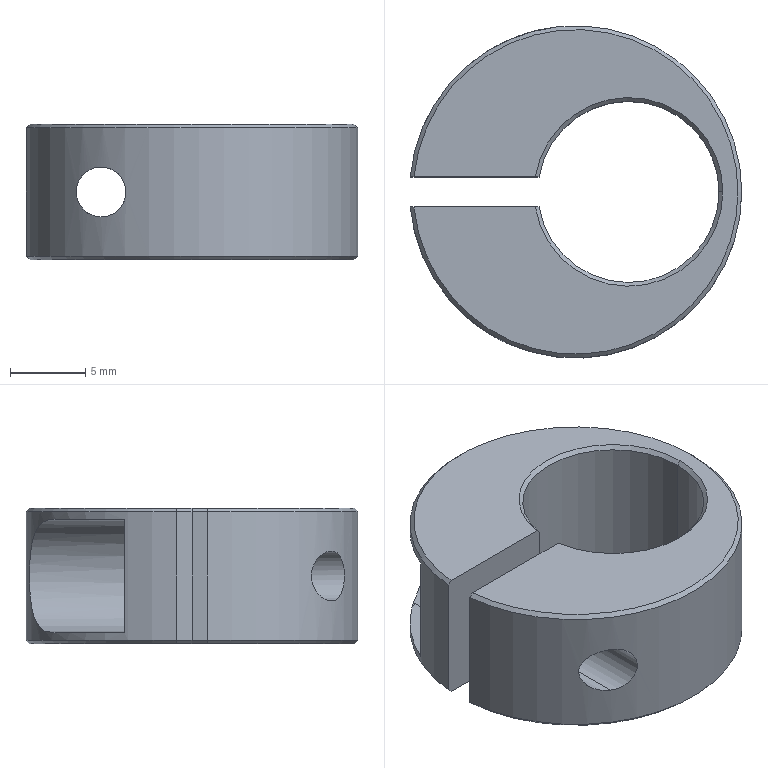Part | NX | features BREP 1 | 1 solid | 25 faces | box 21.954 x 22 x 9 mm | volume 1911 mm3 | cylinder 10 | plane 9 | cone 6 | commonest cylinder face diameters 7.5 x3 3.3 x2 4.5 x2 12 x2 22 x1
STEP:
#1=CARTESIAN_POINT('',(9.5,0.,8.75));
#2=VERTEX_POINT('',#1);
#3=CARTESIAN_POINT('',(9.75,0.,9.));
#4=VERTEX_POINT('',#3);
#5=CARTESIAN_POINT('',(9.5,0.,8.75));
#6=DIRECTION('',(0.7071,0.,0.7071));
#7=VECTOR('',#6,1000.);
#8=LINE('',#5,#7);
#9=EDGE_CURVE('',#2,#4,#8,.T.);
#10=ORIENTED_EDGE('',*,*,#9,.F.);
#11=CARTESIAN_POINT('',(-2.416,-1.,8.75));
#12=VERTEX_POINT('',#11);
#13=CARTESIAN_POINT('',(3.5,0.,8.75));
#14=DIRECTION('',(0.,0.,1.));
#15=DIRECTION('',(1.,0.,0.));
#16=AXIS2_PLACEMENT_3D('',#13,#14,#15);
#17=CIRCLE('',#16,6.);
#18=EDGE_CURVE('',#12,#2,#17,.T.);
#19=ORIENTED_EDGE('',*,*,#18,.F.);
#20=CARTESIAN_POINT('',(-2.669,-1.,9.));
#21=VERTEX_POINT('',#20);
#22=CARTESIAN_POINT('',(-2.669,-1.,9.));
#23=CARTESIAN_POINT('',(-2.585,-1.,8.917));
#24=CARTESIAN_POINT('',(-2.501,-1.,8.833));
#25=CARTESIAN_POINT('',(-2.416,-1.,8.75));
#26=B_SPLINE_CURVE_WITH_KNOTS('',3,(#22,#23,#24,#25),.UNSPECIFIED.,.F.,.F.,(4,4),(0.,0.000356),.UNSPECIFIED.);
#27=EDGE_CURVE('',#21,#12,#26,.T.);
#28=ORIENTED_EDGE('',*,*,#27,.F.);
#29=CARTESIAN_POINT('',(3.5,0.,9.));
#30=DIRECTION('',(0.,0.,-1.));
#31=DIRECTION('',(1.,0.,0.));
#32=AXIS2_PLACEMENT_3D('',#29,#30,#31);
#33=CIRCLE('',#32,6.25);
#34=EDGE_CURVE('',#4,#21,#33,.T.);
#35=ORIENTED_EDGE('',*,*,#34,.F.);
#36=EDGE_LOOP('',(#10,#19,#28,#35));
#37=FACE_BOUND('',#36,.T.);
#38=CARTESIAN_POINT('',(3.5,0.,8.75));
#39=DIRECTION('',(0.,0.,1.));
#40=DIRECTION('',(1.,0.,0.));
#41=AXIS2_PLACEMENT_3D('',#38,#39,#40);
#42=CONICAL_SURFACE('',#41,6.,0.7854);
#43=ADVANCED_FACE('',(#37),#42,.F.);
#44=CARTESIAN_POINT('',(-10.954,-1.,8.75));
#45=VERTEX_POINT('',#44);
#46=CARTESIAN_POINT('',(-10.703,-1.,9.));
#47=VERTEX_POINT('',#46);
#48=CARTESIAN_POINT('',(-10.954,-1.,8.75));
#49=CARTESIAN_POINT('',(-10.871,-1.,8.833));
#50=CARTESIAN_POINT('',(-10.787,-1.,8.917));
#51=CARTESIAN_POINT('',(-10.703,-1.,9.));
#52=B_SPLINE_CURVE_WITH_KNOTS('',3,(#48,#49,#50,#51),.UNSPECIFIED.,.F.,.F.,(4,4),(0.,0.0003543),.UNSPECIFIED.);
#53=EDGE_CURVE('',#45,#47,#52,.T.);
#54=ORIENTED_EDGE('',*,*,#53,.F.);
#55=CARTESIAN_POINT('',(-10.954,1.,8.75));
#56=VERTEX_POINT('',#55);
#57=CARTESIAN_POINT('',(0.,0.,8.75));
#58=DIRECTION('',(0.,0.,-1.));
#59=DIRECTION('',(1.,0.,0.));
#60=AXIS2_PLACEMENT_3D('',#57,#58,#59);
#61=CIRCLE('',#60,11.);
#62=EDGE_CURVE('',#56,#45,#61,.T.);
#63=ORIENTED_EDGE('',*,*,#62,.F.);
#64=CARTESIAN_POINT('',(-10.703,1.,9.));
#65=VERTEX_POINT('',#64);
#66=CARTESIAN_POINT('',(-10.703,1.,9.));
#67=CARTESIAN_POINT('',(-10.787,1.,8.917));
#68=CARTESIAN_POINT('',(-10.871,1.,8.833));
#69=CARTESIAN_POINT('',(-10.954,1.,8.75));
#70=B_SPLINE_CURVE_WITH_KNOTS('',3,(#66,#67,#68,#69),.UNSPECIFIED.,.F.,.F.,(4,4),(0.,0.0003543),.UNSPECIFIED.);
#71=EDGE_CURVE('',#65,#56,#70,.T.);
#72=ORIENTED_EDGE('',*,*,#71,.F.);
#73=CARTESIAN_POINT('',(0.,0.,9.));
#74=DIRECTION('',(0.,0.,1.));
#75=DIRECTION('',(1.,0.,0.));
#76=AXIS2_PLACEMENT_3D('',#73,#74,#75);
#77=CIRCLE('',#76,10.75);
#78=EDGE_CURVE('',#47,#65,#77,.T.);
#79=ORIENTED_EDGE('',*,*,#78,.F.);
#80=EDGE_LOOP('',(#54,#63,#72,#79));
#81=FACE_BOUND('',#80,.T.);
#82=CARTESIAN_POINT('',(0.,0.,9.));
#83=DIRECTION('',(0.,0.,-1.));
#84=DIRECTION('',(-1.,0.,0.));
#85=AXIS2_PLACEMENT_3D('',#82,#83,#84);
#86=CONICAL_SURFACE('',#85,10.75,0.7854);
#87=ADVANCED_FACE('',(#81),#86,.T.);
#88=CARTESIAN_POINT('',(-2.669,1.,0.));
#89=VERTEX_POINT('',#88);
#90=CARTESIAN_POINT('',(-2.416,1.,0.25));
#91=VERTEX_POINT('',#90);
#92=CARTESIAN_POINT('',(-2.669,1.,0.));
#93=CARTESIAN_POINT('',(-2.585,1.,0.08336));
#94=CARTESIAN_POINT('',(-2.501,1.,0.1667));
#95=CARTESIAN_POINT('',(-2.416,1.,0.25));
#96=B_SPLINE_CURVE_WITH_KNOTS('',3,(#92,#93,#94,#95),.UNSPECIFIED.,.F.,.F.,(4,4),(0.,0.000356),.UNSPECIFIED.);
#97=EDGE_CURVE('',#89,#91,#96,.T.);
#98=ORIENTED_EDGE('',*,*,#97,.F.);
#99=CARTESIAN_POINT('',(-2.669,-1.,0.));
#100=VERTEX_POINT('',#99);
#101=CARTESIAN_POINT('',(3.5,0.,0.));
#102=DIRECTION('',(0.,0.,1.));
#103=DIRECTION('',(1.,0.,0.));
#104=AXIS2_PLACEMENT_3D('',#101,#102,#103);
#105=CIRCLE('',#104,6.25);
#106=EDGE_CURVE('',#100,#89,#105,.T.);
#107=ORIENTED_EDGE('',*,*,#106,.F.);
#108=CARTESIAN_POINT('',(-2.416,-1.,0.25));
#109=VERTEX_POINT('',#108);
#110=CARTESIAN_POINT('',(-2.416,-1.,0.25));
#111=CARTESIAN_POINT('',(-2.501,-1.,0.1667));
#112=CARTESIAN_POINT('',(-2.585,-1.,0.08336));
#113=CARTESIAN_POINT('',(-2.669,-1.,0.));
#114=B_SPLINE_CURVE_WITH_KNOTS('',3,(#110,#111,#112,#113),.UNSPECIFIED.,.F.,.F.,(4,4),(0.,0.000356),.UNSPECIFIED.);
#115=EDGE_CURVE('',#109,#100,#114,.T.);
#116=ORIENTED_EDGE('',*,*,#115,.F.);
#117=CARTESIAN_POINT('',(9.5,0.,0.25));
#118=VERTEX_POINT('',#117);
#119=CARTESIAN_POINT('',(3.5,0.,0.25));
#120=DIRECTION('',(0.,0.,-1.));
#121=DIRECTION('',(1.,0.,0.));
#122=AXIS2_PLACEMENT_3D('',#119,#120,#121);
#123=CIRCLE('',#122,6.);
#124=EDGE_CURVE('',#118,#109,#123,.T.);
#125=ORIENTED_EDGE('',*,*,#124,.F.);
#126=CARTESIAN_POINT('',(3.5,0.,0.25));
#127=DIRECTION('',(0.,0.,-1.));
#128=DIRECTION('',(1.,0.,0.));
#129=AXIS2_PLACEMENT_3D('',#126,#127,#128);
#130=CIRCLE('',#129,6.);
#131=EDGE_CURVE('',#91,#118,#130,.T.);
#132=ORIENTED_EDGE('',*,*,#131,.F.);
#133=EDGE_LOOP('',(#98,#107,#116,#125,#132));
#134=FACE_BOUND('',#133,.T.);
#135=CARTESIAN_POINT('',(3.5,0.,0.25));
#136=DIRECTION('',(0.,0.,-1.));
#137=DIRECTION('',(-1.,0.,0.));
#138=AXIS2_PLACEMENT_3D('',#135,#136,#137);
#139=CONICAL_SURFACE('',#138,6.,0.7854);
#140=ADVANCED_FACE('',(#134),#139,.F.);
#141=CARTESIAN_POINT('',(10.75,0.,0.));
#142=VERTEX_POINT('',#141);
#143=CARTESIAN_POINT('',(11.,0.,0.25));
#144=VERTEX_POINT('',#143);
#145=CARTESIAN_POINT('',(11.,0.,0.25));
#146=DIRECTION('',(0.7071,0.,0.7071));
#147=VECTOR('',#146,1000.);
#148=LINE('',#145,#147);
#149=EDGE_CURVE('',#142,#144,#148,.T.);
#150=ORIENTED_EDGE('',*,*,#149,.F.);
#151=CARTESIAN_POINT('',(-10.703,1.,0.));
#152=VERTEX_POINT('',#151);
#153=CARTESIAN_POINT('',(0.,0.,0.));
#154=DIRECTION('',(0.,0.,-1.));
#155=DIRECTION('',(1.,0.,0.));
#156=AXIS2_PLACEMENT_3D('',#153,#154,#155);
#157=CIRCLE('',#156,10.75);
#158=EDGE_CURVE('',#152,#142,#157,.T.);
#159=ORIENTED_EDGE('',*,*,#158,.F.);
#160=CARTESIAN_POINT('',(-10.954,1.,0.25));
#161=VERTEX_POINT('',#160);
#162=CARTESIAN_POINT('',(-10.954,1.,0.25));
#163=CARTESIAN_POINT('',(-10.871,1.,0.1667));
#164=CARTESIAN_POINT('',(-10.787,1.,0.08333));
#165=CARTESIAN_POINT('',(-10.703,1.,0.));
#166=B_SPLINE_CURVE_WITH_KNOTS('',3,(#162,#163,#164,#165),.UNSPECIFIED.,.F.,.F.,(4,4),(0.,0.0003543),.UNSPECIFIED.);
#167=EDGE_CURVE('',#161,#152,#166,.T.);
#168=ORIENTED_EDGE('',*,*,#167,.F.);
#169=CARTESIAN_POINT('',(0.,0.,0.25));
#170=DIRECTION('',(0.,0.,1.));
#171=DIRECTION('',(1.,0.,0.));
#172=AXIS2_PLACEMENT_3D('',#169,#170,#171);
#173=CIRCLE('',#172,11.);
#174=EDGE_CURVE('',#144,#161,#173,.T.);
#175=ORIENTED_EDGE('',*,*,#174,.F.);
#176=EDGE_LOOP('',(#150,#159,#168,#175));
#177=FACE_BOUND('',#176,.T.);
#178=CARTESIAN_POINT('',(0.,0.,0.25));
#179=DIRECTION('',(0.,0.,1.));
#180=DIRECTION('',(1.,0.,0.));
#181=AXIS2_PLACEMENT_3D('',#178,#179,#180);
#182=CONICAL_SURFACE('',#181,11.,0.7854);
#183=ADVANCED_FACE('',(#177),#182,.T.);
#184=CARTESIAN_POINT('',(-6.,-1.,2.85));
#185=VERTEX_POINT('',#184);
#186=CARTESIAN_POINT('',(-6.,-9.22,2.85));
#187=VERTEX_POINT('',#186);
#188=CARTESIAN_POINT('',(-6.,-1.,2.85));
#189=DIRECTION('',(0.,1.,0.));
#190=VECTOR('',#189,1000.);
#191=LINE('',#188,#190);
#192=EDGE_CURVE('',#185,#187,#191,.F.);
#193=ORIENTED_EDGE('',*,*,#192,.T.);
#194=CARTESIAN_POINT('',(-6.,-9.22,6.15));
#195=VERTEX_POINT('',#194);
#196=CARTESIAN_POINT('',(-6.,-9.22,2.85));
#197=CARTESIAN_POINT('',(-5.573,-9.497,2.85));
#198=CARTESIAN_POINT('',(-4.796,-9.917,3.131));
#199=CARTESIAN_POINT('',(-4.125,-10.197,4.506));
#200=CARTESIAN_POINT('',(-4.804,-9.914,5.873));
#201=CARTESIAN_POINT('',(-5.574,-9.496,6.15));
#202=CARTESIAN_POINT('',(-6.,-9.22,6.15));
#203=B_SPLINE_CURVE_WITH_KNOTS('',3,(#196,#197,#198,#199,#200,#201,#202),.UNSPECIFIED.,.F.,.F.,(4,1,1,1,4),(0.,0.25,0.5,0.75,1.),.UNSPECIFIED.);
#204=EDGE_CURVE('',#195,#187,#203,.F.);
#205=ORIENTED_EDGE('',*,*,#204,.F.);
#206=CARTESIAN_POINT('',(-6.,-1.,6.15));
#207=VERTEX_POINT('',#206);
#208=CARTESIAN_POINT('',(-6.,-1.,6.15));
#209=DIRECTION('',(0.,1.,0.));
#210=VECTOR('',#209,1000.);
#211=LINE('',#208,#210);
#212=EDGE_CURVE('',#207,#195,#211,.F.);
#213=ORIENTED_EDGE('',*,*,#212,.F.);
#214=CARTESIAN_POINT('',(-6.,-1.,4.5));
#215=DIRECTION('',(0.,1.,0.));
#216=DIRECTION('',(0.,0.,1.));
#217=AXIS2_PLACEMENT_3D('',#214,#215,#216);
#218=CIRCLE('',#217,1.65);
#219=EDGE_CURVE('',#207,#185,#218,.T.);
#220=ORIENTED_EDGE('',*,*,#219,.T.);
#221=EDGE_LOOP('',(#193,#205,#213,#220));
#222=FACE_BOUND('',#221,.T.);
#223=CARTESIAN_POINT('',(-6.,-1.,4.5));
#224=DIRECTION('',(0.,1.,0.));
#225=DIRECTION('',(0.,0.,1.));
#226=AXIS2_PLACEMENT_3D('',#223,#224,#225);
#227=CYLINDRICAL_SURFACE('',#226,1.65);
#228=ADVANCED_FACE('',(#222),#227,.F.);
#229=CARTESIAN_POINT('',(-6.325,9.,8.25));
#230=VERTEX_POINT('',#229);
#231=CARTESIAN_POINT('',(-6.325,9.,8.236));
#232=VERTEX_POINT('',#231);
#233=CARTESIAN_POINT('',(-6.325,9.,9.));
#234=DIRECTION('',(0.,0.,-1.));
#235=VECTOR('',#234,1000.);
#236=LINE('',#233,#235);
#237=EDGE_CURVE('',#230,#232,#236,.T.);
#238=ORIENTED_EDGE('',*,*,#237,.T.);
#239=CARTESIAN_POINT('',(-6.,9.,8.25));
#240=VERTEX_POINT('',#239);
#241=CARTESIAN_POINT('',(-6.,9.,4.5));
#242=DIRECTION('',(0.,1.,0.));
#243=DIRECTION('',(0.,0.,-1.));
#244=AXIS2_PLACEMENT_3D('',#241,#242,#243);
#245=CIRCLE('',#244,3.75);
#246=EDGE_CURVE('',#232,#240,#245,.T.);
#247=ORIENTED_EDGE('',*,*,#246,.T.);
#248=CARTESIAN_POINT('',(-6.,9.,8.25));
#249=DIRECTION('',(1.,0.,0.));
#250=VECTOR('',#249,1000.);
#251=LINE('',#248,#250);
#252=EDGE_CURVE('',#230,#240,#251,.T.);
#253=ORIENTED_EDGE('',*,*,#252,.F.);
#254=EDGE_LOOP('',(#238,#247,#253));
#255=FACE_BOUND('',#254,.T.);
#256=CARTESIAN_POINT('',(0.,9.,0.));
#257=DIRECTION('',(0.,-1.,0.));
#258=DIRECTION('',(0.,0.,-1.));
#259=AXIS2_PLACEMENT_3D('',#256,#257,#258);
#260=PLANE('',#259);
#261=ADVANCED_FACE('',(#255),#260,.T.);
#262=CARTESIAN_POINT('',(-6.325,9.,0.7641));
#263=VERTEX_POINT('',#262);
#264=CARTESIAN_POINT('',(-6.325,9.,0.75));
#265=VERTEX_POINT('',#264);
#266=CARTESIAN_POINT('',(-6.325,9.,9.));
#267=DIRECTION('',(0.,0.,-1.));
#268=VECTOR('',#267,1000.);
#269=LINE('',#266,#268);
#270=EDGE_CURVE('',#263,#265,#269,.T.);
#271=ORIENTED_EDGE('',*,*,#270,.T.);
#272=CARTESIAN_POINT('',(-6.,9.,0.75));
#273=VERTEX_POINT('',#272);
#274=CARTESIAN_POINT('',(-6.,9.,0.75));
#275=DIRECTION('',(-1.,0.,0.));
#276=VECTOR('',#275,1000.);
#277=LINE('',#274,#276);
#278=EDGE_CURVE('',#273,#265,#277,.T.);
#279=ORIENTED_EDGE('',*,*,#278,.F.);
#280=CARTESIAN_POINT('',(-6.,9.,4.5));
#281=DIRECTION('',(0.,1.,0.));
#282=DIRECTION('',(0.,0.,-1.));
#283=AXIS2_PLACEMENT_3D('',#280,#281,#282);
#284=CIRCLE('',#283,3.75);
#285=EDGE_CURVE('',#273,#263,#284,.T.);
#286=ORIENTED_EDGE('',*,*,#285,.T.);
#287=EDGE_LOOP('',(#271,#279,#286));
#288=FACE_BOUND('',#287,.T.);
#289=CARTESIAN_POINT('',(0.,9.,0.));
#290=DIRECTION('',(0.,-1.,0.));
#291=DIRECTION('',(0.,0.,-1.));
#292=AXIS2_PLACEMENT_3D('',#289,#290,#291);
#293=PLANE('',#292);
#294=ADVANCED_FACE('',(#288),#293,.T.);
#295=CARTESIAN_POINT('',(-10.037,4.5,0.75));
#296=VERTEX_POINT('',#295);
#297=CARTESIAN_POINT('',(0.,0.,0.75));
#298=DIRECTION('',(0.,0.,1.));
#299=DIRECTION('',(1.,0.,0.));
#300=AXIS2_PLACEMENT_3D('',#297,#298,#299);
#301=CIRCLE('',#300,11.);
#302=EDGE_CURVE('',#265,#296,#301,.T.);
#303=ORIENTED_EDGE('',*,*,#302,.T.);
#304=CARTESIAN_POINT('',(-6.,4.5,0.75));
#305=VERTEX_POINT('',#304);
#306=CARTESIAN_POINT('',(-6.,4.5,0.75));
#307=DIRECTION('',(-1.,0.,0.));
#308=VECTOR('',#307,1000.);
#309=LINE('',#306,#308);
#310=EDGE_CURVE('',#305,#296,#309,.T.);
#311=ORIENTED_EDGE('',*,*,#310,.F.);
#312=CARTESIAN_POINT('',(-6.,9.,0.75));
#313=DIRECTION('',(0.,-1.,0.));
#314=VECTOR('',#313,1000.);
#315=LINE('',#312,#314);
#316=EDGE_CURVE('',#273,#305,#315,.T.);
#317=ORIENTED_EDGE('',*,*,#316,.F.);
#318=ORIENTED_EDGE('',*,*,#278,.T.);
#319=EDGE_LOOP('',(#303,#311,#317,#318));
#320=FACE_BOUND('',#319,.T.);
#321=CARTESIAN_POINT('',(-6.,9.,0.75));
#322=DIRECTION('',(0.,0.,1.));
#323=DIRECTION('',(1.,0.,0.));
#324=AXIS2_PLACEMENT_3D('',#321,#322,#323);
#325=PLANE('',#324);
#326=ADVANCED_FACE('',(#320),#325,.T.);
#327=CARTESIAN_POINT('',(-10.037,4.5,8.25));
#328=VERTEX_POINT('',#327);
#329=CARTESIAN_POINT('',(0.,0.,8.25));
#330=DIRECTION('',(0.,0.,-1.));
#331=DIRECTION('',(-1.,0.,0.));
#332=AXIS2_PLACEMENT_3D('',#329,#330,#331);
#333=CIRCLE('',#332,11.);
#334=EDGE_CURVE('',#328,#230,#333,.T.);
#335=ORIENTED_EDGE('',*,*,#334,.T.);
#336=ORIENTED_EDGE('',*,*,#252,.T.);
#337=CARTESIAN_POINT('',(-6.,4.5,8.25));
#338=VERTEX_POINT('',#337);
#339=CARTESIAN_POINT('',(-6.,9.,8.25));
#340=DIRECTION('',(0.,-1.,0.));
#341=VECTOR('',#340,1000.);
#342=LINE('',#339,#341);
#343=EDGE_CURVE('',#240,#338,#342,.T.);
#344=ORIENTED_EDGE('',*,*,#343,.T.);
#345=CARTESIAN_POINT('',(-6.,4.5,8.25));
#346=DIRECTION('',(1.,0.,0.));
#347=VECTOR('',#346,1000.);
#348=LINE('',#345,#347);
#349=EDGE_CURVE('',#328,#338,#348,.T.);
#350=ORIENTED_EDGE('',*,*,#349,.F.);
#351=EDGE_LOOP('',(#335,#336,#344,#350));
#352=FACE_BOUND('',#351,.T.);
#353=CARTESIAN_POINT('',(-6.,9.,8.25));
#354=DIRECTION('',(0.,0.,-1.));
#355=DIRECTION('',(-1.,0.,0.));
#356=AXIS2_PLACEMENT_3D('',#353,#354,#355);
#357=PLANE('',#356);
#358=ADVANCED_FACE('',(#352),#357,.T.);
#359=ORIENTED_EDGE('',*,*,#349,.T.);
#360=CARTESIAN_POINT('',(-6.,4.5,4.5));
#361=DIRECTION('',(0.,-1.,0.));
#362=DIRECTION('',(0.,0.,-1.));
#363=AXIS2_PLACEMENT_3D('',#360,#361,#362);
#364=CIRCLE('',#363,3.75);
#365=EDGE_CURVE('',#305,#338,#364,.T.);
#366=ORIENTED_EDGE('',*,*,#365,.F.);
#367=ORIENTED_EDGE('',*,*,#310,.T.);
#368=CARTESIAN_POINT('',(-10.037,4.5,9.));
#369=DIRECTION('',(0.,0.,-1.));
#370=VECTOR('',#369,1000.);
#371=LINE('',#368,#370);
#372=EDGE_CURVE('',#328,#296,#371,.T.);
#373=ORIENTED_EDGE('',*,*,#372,.F.);
#374=EDGE_LOOP('',(#359,#366,#367,#373));
#375=FACE_BOUND('',#374,.T.);
#376=CARTESIAN_POINT('',(-6.,4.5,2.25));
#377=VERTEX_POINT('',#376);
#378=CARTESIAN_POINT('',(-6.,4.5,6.75));
#379=VERTEX_POINT('',#378);
#380=CARTESIAN_POINT('',(-6.,4.5,4.5));
#381=DIRECTION('',(0.,1.,0.));
#382=DIRECTION('',(0.,0.,-1.));
#383=AXIS2_PLACEMENT_3D('',#380,#381,#382);
#384=CIRCLE('',#383,2.25);
#385=EDGE_CURVE('',#377,#379,#384,.T.);
#386=ORIENTED_EDGE('',*,*,#385,.F.);
#387=CARTESIAN_POINT('',(-6.,4.5,4.5));
#388=DIRECTION('',(0.,1.,0.));
#389=DIRECTION('',(0.,0.,-1.));
#390=AXIS2_PLACEMENT_3D('',#387,#388,#389);
#391=CIRCLE('',#390,2.25);
#392=EDGE_CURVE('',#379,#377,#391,.T.);
#393=ORIENTED_EDGE('',*,*,#392,.F.);
#394=EDGE_LOOP('',(#386,#393));
#395=FACE_BOUND('',#394,.T.);
#396=CARTESIAN_POINT('',(-6.,4.5,4.5));
#397=DIRECTION('',(0.,-1.,0.));
#398=DIRECTION('',(0.,0.,-1.));
#399=AXIS2_PLACEMENT_3D('',#396,#397,#398);
#400=PLANE('',#399);
#401=ADVANCED_FACE('',(#375,#395),#400,.F.);
#402=CARTESIAN_POINT('',(-6.,1.,6.75));
#403=VERTEX_POINT('',#402);
#404=CARTESIAN_POINT('',(-6.,4.5,6.75));
#405=DIRECTION('',(0.,-1.,0.));
#406=VECTOR('',#405,1000.);
#407=LINE('',#404,#406);
#408=EDGE_CURVE('',#379,#403,#407,.T.);
#409=ORIENTED_EDGE('',*,*,#408,.F.);
#410=ORIENTED_EDGE('',*,*,#392,.T.);
#411=CARTESIAN_POINT('',(-6.,1.,2.25));
#412=VERTEX_POINT('',#411);
#413=CARTESIAN_POINT('',(-6.,4.5,2.25));
#414=DIRECTION('',(0.,-1.,0.));
#415=VECTOR('',#414,1000.);
#416=LINE('',#413,#415);
#417=EDGE_CURVE('',#377,#412,#416,.T.);
#418=ORIENTED_EDGE('',*,*,#417,.T.);
#419=CARTESIAN_POINT('',(-6.,1.,4.5));
#420=DIRECTION('',(0.,-1.,0.));
#421=DIRECTION('',(0.,0.,-1.));
#422=AXIS2_PLACEMENT_3D('',#419,#420,#421);
#423=CIRCLE('',#422,2.25);
#424=EDGE_CURVE('',#412,#403,#423,.T.);
#425=ORIENTED_EDGE('',*,*,#424,.T.);
#426=EDGE_LOOP('',(#409,#410,#418,#425));
#427=FACE_BOUND('',#426,.T.);
#428=CARTESIAN_POINT('',(-6.,4.5,4.5));
#429=DIRECTION('',(0.,-1.,0.));
#430=DIRECTION('',(0.,0.,-1.));
#431=AXIS2_PLACEMENT_3D('',#428,#429,#430);
#432=CYLINDRICAL_SURFACE('',#431,2.25);
#433=ADVANCED_FACE('',(#427),#432,.F.);
#434=CARTESIAN_POINT('',(-10.703,-1.,0.));
#435=VERTEX_POINT('',#434);
#436=CARTESIAN_POINT('',(-19.584,-1.,0.));
#437=DIRECTION('',(-1.,0.,0.));
#438=VECTOR('',#437,1000.);
#439=LINE('',#436,#438);
#440=EDGE_CURVE('',#100,#435,#439,.T.);
#441=ORIENTED_EDGE('',*,*,#440,.T.);
#442=CARTESIAN_POINT('',(-10.954,-1.,0.25));
#443=VERTEX_POINT('',#442);
#444=CARTESIAN_POINT('',(-10.703,-1.,0.));
#445=CARTESIAN_POINT('',(-10.787,-1.,0.08333));
#446=CARTESIAN_POINT('',(-10.871,-1.,0.1667));
#447=CARTESIAN_POINT('',(-10.954,-1.,0.25));
#448=B_SPLINE_CURVE_WITH_KNOTS('',3,(#444,#445,#446,#447),.UNSPECIFIED.,.F.,.F.,(4,4),(0.,0.0003543),.UNSPECIFIED.);
#449=EDGE_CURVE('',#435,#443,#448,.T.);
#450=ORIENTED_EDGE('',*,*,#449,.T.);
#451=CARTESIAN_POINT('',(-10.954,-1.,9.));
#452=DIRECTION('',(0.,0.,1.));
#453=VECTOR('',#452,1000.);
#454=LINE('',#451,#453);
#455=EDGE_CURVE('',#443,#45,#454,.T.);
#456=ORIENTED_EDGE('',*,*,#455,.T.);
#457=ORIENTED_EDGE('',*,*,#53,.T.);
#458=CARTESIAN_POINT('',(-19.584,-1.,9.));
#459=DIRECTION('',(1.,0.,0.));
#460=VECTOR('',#459,1000.);
#461=LINE('',#458,#460);
#462=EDGE_CURVE('',#47,#21,#461,.T.);
#463=ORIENTED_EDGE('',*,*,#462,.T.);
#464=ORIENTED_EDGE('',*,*,#27,.T.);
#465=CARTESIAN_POINT('',(-2.416,-1.,-0.001));
#466=DIRECTION('',(0.,0.,-1.));
#467=VECTOR('',#466,1000.);
#468=LINE('',#465,#467);
#469=EDGE_CURVE('',#12,#109,#468,.T.);
#470=ORIENTED_EDGE('',*,*,#469,.T.);
#471=ORIENTED_EDGE('',*,*,#115,.T.);
#472=EDGE_LOOP('',(#441,#450,#456,#457,#463,#464,#470,#471));
#473=FACE_BOUND('',#472,.T.);
#474=ORIENTED_EDGE('',*,*,#219,.F.);
#475=CARTESIAN_POINT('',(-6.,-1.,4.5));
#476=DIRECTION('',(0.,1.,0.));
#477=DIRECTION('',(0.,0.,1.));
#478=AXIS2_PLACEMENT_3D('',#475,#476,#477);
#479=CIRCLE('',#478,1.65);
#480=EDGE_CURVE('',#185,#207,#479,.T.);
#481=ORIENTED_EDGE('',*,*,#480,.F.);
#482=EDGE_LOOP('',(#474,#481));
#483=FACE_BOUND('',#482,.T.);
#484=CARTESIAN_POINT('',(-19.584,-1.,-0.001));
#485=DIRECTION('',(0.,-1.,0.));
#486=DIRECTION('',(0.,0.,-1.));
#487=AXIS2_PLACEMENT_3D('',#484,#485,#486);
#488=PLANE('',#487);
#489=ADVANCED_FACE('',(#473,#483),#488,.F.);
#490=CARTESIAN_POINT('',(-10.954,1.,9.));
#491=DIRECTION('',(0.,0.,-1.));
#492=VECTOR('',#491,1000.);
#493=LINE('',#490,#492);
#494=EDGE_CURVE('',#56,#161,#493,.T.);
#495=ORIENTED_EDGE('',*,*,#494,.T.);
#496=ORIENTED_EDGE('',*,*,#167,.T.);
#497=CARTESIAN_POINT('',(-19.584,1.,0.));
#498=DIRECTION('',(1.,0.,0.));
#499=VECTOR('',#498,1000.);
#500=LINE('',#497,#499);
#501=EDGE_CURVE('',#152,#89,#500,.T.);
#502=ORIENTED_EDGE('',*,*,#501,.T.);
#503=ORIENTED_EDGE('',*,*,#97,.T.);
#504=CARTESIAN_POINT('',(-2.416,1.,8.75));
#505=VERTEX_POINT('',#504);
#506=CARTESIAN_POINT('',(-2.416,1.,-0.001));
#507=DIRECTION('',(0.,0.,1.));
#508=VECTOR('',#507,1000.);
#509=LINE('',#506,#508);
#510=EDGE_CURVE('',#91,#505,#509,.T.);
#511=ORIENTED_EDGE('',*,*,#510,.T.);
#512=CARTESIAN_POINT('',(-2.669,1.,9.));
#513=VERTEX_POINT('',#512);
#514=CARTESIAN_POINT('',(-2.416,1.,8.75));
#515=CARTESIAN_POINT('',(-2.501,1.,8.833));
#516=CARTESIAN_POINT('',(-2.585,1.,8.917));
#517=CARTESIAN_POINT('',(-2.669,1.,9.));
#518=B_SPLINE_CURVE_WITH_KNOTS('',3,(#514,#515,#516,#517),.UNSPECIFIED.,.F.,.F.,(4,4),(0.,0.000356),.UNSPECIFIED.);
#519=EDGE_CURVE('',#505,#513,#518,.T.);
#520=ORIENTED_EDGE('',*,*,#519,.T.);
#521=CARTESIAN_POINT('',(-19.584,1.,9.));
#522=DIRECTION('',(-1.,0.,0.));
#523=VECTOR('',#522,1000.);
#524=LINE('',#521,#523);
#525=EDGE_CURVE('',#513,#65,#524,.T.);
#526=ORIENTED_EDGE('',*,*,#525,.T.);
#527=ORIENTED_EDGE('',*,*,#71,.T.);
#528=EDGE_LOOP('',(#495,#496,#502,#503,#511,#520,#526,#527));
#529=FACE_BOUND('',#528,.T.);
#530=ORIENTED_EDGE('',*,*,#424,.F.);
#531=CARTESIAN_POINT('',(-6.,1.,4.5));
#532=DIRECTION('',(0.,-1.,0.));
#533=DIRECTION('',(0.,0.,-1.));
#534=AXIS2_PLACEMENT_3D('',#531,#532,#533);
#535=CIRCLE('',#534,2.25);
#536=EDGE_CURVE('',#403,#412,#535,.T.);
#537=ORIENTED_EDGE('',*,*,#536,.F.);
#538=EDGE_LOOP('',(#530,#537));
#539=FACE_BOUND('',#538,.T.);
#540=CARTESIAN_POINT('',(-19.584,1.,-0.001));
#541=DIRECTION('',(0.,1.,0.));
#542=DIRECTION('',(0.,0.,1.));
#543=AXIS2_PLACEMENT_3D('',#540,#541,#542);
#544=PLANE('',#543);
#545=ADVANCED_FACE('',(#529,#539),#544,.F.);
#546=CARTESIAN_POINT('',(9.5,0.,-0.001));
#547=DIRECTION('',(0.,0.,1.));
#548=VECTOR('',#547,1000.);
#549=LINE('',#546,#548);
#550=EDGE_CURVE('',#118,#2,#549,.T.);
#551=ORIENTED_EDGE('',*,*,#550,.F.);
#552=ORIENTED_EDGE('',*,*,#124,.T.);
#553=ORIENTED_EDGE('',*,*,#469,.F.);
#554=ORIENTED_EDGE('',*,*,#18,.T.);
#555=EDGE_LOOP('',(#551,#552,#553,#554));
#556=FACE_BOUND('',#555,.T.);
#557=CARTESIAN_POINT('',(3.5,0.,-0.001));
#558=DIRECTION('',(0.,0.,1.));
#559=DIRECTION('',(1.,0.,0.));
#560=AXIS2_PLACEMENT_3D('',#557,#558,#559);
#561=CYLINDRICAL_SURFACE('',#560,6.);
#562=ADVANCED_FACE('',(#556),#561,.F.);
#563=ORIENTED_EDGE('',*,*,#501,.F.);
#564=ORIENTED_EDGE('',*,*,#158,.T.);
#565=CARTESIAN_POINT('',(0.,0.,0.));
#566=DIRECTION('',(0.,0.,-1.));
#567=DIRECTION('',(1.,0.,0.));
#568=AXIS2_PLACEMENT_3D('',#565,#566,#567);
#569=CIRCLE('',#568,10.75);
#570=EDGE_CURVE('',#142,#435,#569,.T.);
#571=ORIENTED_EDGE('',*,*,#570,.T.);
#572=ORIENTED_EDGE('',*,*,#440,.F.);
#573=ORIENTED_EDGE('',*,*,#106,.T.);
#574=EDGE_LOOP('',(#563,#564,#571,#572,#573));
#575=FACE_BOUND('',#574,.T.);
#576=CARTESIAN_POINT('',(0.,0.,0.));
#577=DIRECTION('',(0.,0.,1.));
#578=DIRECTION('',(1.,0.,0.));
#579=AXIS2_PLACEMENT_3D('',#576,#577,#578);
#580=PLANE('',#579);
#581=ADVANCED_FACE('',(#575),#580,.F.);
#582=ORIENTED_EDGE('',*,*,#462,.F.);
#583=ORIENTED_EDGE('',*,*,#78,.T.);
#584=ORIENTED_EDGE('',*,*,#525,.F.);
#585=CARTESIAN_POINT('',(3.5,0.,9.));
#586=DIRECTION('',(0.,0.,-1.));
#587=DIRECTION('',(1.,0.,0.));
#588=AXIS2_PLACEMENT_3D('',#585,#586,#587);
#589=CIRCLE('',#588,6.25);
#590=EDGE_CURVE('',#513,#4,#589,.T.);
#591=ORIENTED_EDGE('',*,*,#590,.T.);
#592=ORIENTED_EDGE('',*,*,#34,.T.);
#593=EDGE_LOOP('',(#582,#583,#584,#591,#592));
#594=FACE_BOUND('',#593,.T.);
#595=CARTESIAN_POINT('',(0.,0.,9.));
#596=DIRECTION('',(0.,0.,1.));
#597=DIRECTION('',(1.,0.,0.));
#598=AXIS2_PLACEMENT_3D('',#595,#596,#597);
#599=PLANE('',#598);
#600=ADVANCED_FACE('',(#594),#599,.T.);
#601=CARTESIAN_POINT('',(-6.,9.22,0.75));
#602=VERTEX_POINT('',#601);
#603=CARTESIAN_POINT('',(-6.,11.001,0.75));
#604=DIRECTION('',(0.,-1.,0.));
#605=VECTOR('',#604,1000.);
#606=LINE('',#603,#605);
#607=EDGE_CURVE('',#602,#273,#606,.T.);
#608=ORIENTED_EDGE('',*,*,#607,.F.);
#609=CARTESIAN_POINT('',(-6.,9.22,0.75));
#610=CARTESIAN_POINT('',(-6.055,9.184,0.75));
#611=CARTESIAN_POINT('',(-6.164,9.111,0.7524));
#612=CARTESIAN_POINT('',(-6.271,9.037,0.7595));
#613=CARTESIAN_POINT('',(-6.325,9.,0.7641));
#614=B_SPLINE_CURVE_WITH_KNOTS('',3,(#609,#610,#611,#612,#613),.UNSPECIFIED.,.F.,.F.,(4,1,4),(0.,0.0001941,0.0003881),.UNSPECIFIED.);
#615=EDGE_CURVE('',#602,#263,#614,.T.);
#616=ORIENTED_EDGE('',*,*,#615,.T.);
#617=ORIENTED_EDGE('',*,*,#285,.F.);
#618=EDGE_LOOP('',(#608,#616,#617));
#619=FACE_BOUND('',#618,.T.);
#620=CARTESIAN_POINT('',(-6.,11.001,4.5));
#621=DIRECTION('',(0.,-1.,0.));
#622=DIRECTION('',(0.,0.,-1.));
#623=AXIS2_PLACEMENT_3D('',#620,#621,#622);
#624=CYLINDRICAL_SURFACE('',#623,3.75);
#625=ADVANCED_FACE('',(#619),#624,.F.);
#626=ORIENTED_EDGE('',*,*,#237,.F.);
#627=ORIENTED_EDGE('',*,*,#334,.F.);
#628=ORIENTED_EDGE('',*,*,#372,.T.);
#629=ORIENTED_EDGE('',*,*,#302,.F.);
#630=ORIENTED_EDGE('',*,*,#270,.F.);
#631=ORIENTED_EDGE('',*,*,#615,.F.);
#632=CARTESIAN_POINT('',(-6.,9.22,8.25));
#633=VERTEX_POINT('',#632);
#634=CARTESIAN_POINT('',(-6.,9.22,0.75));
#635=CARTESIAN_POINT('',(-5.545,9.516,0.75));
#636=CARTESIAN_POINT('',(-4.665,9.999,0.9032));
#637=CARTESIAN_POINT('',(-2.933,10.658,1.939));
#638=CARTESIAN_POINT('',(-1.791,10.841,4.511));
#639=CARTESIAN_POINT('',(-2.943,10.655,7.071));
#640=CARTESIAN_POINT('',(-4.672,9.995,8.099));
#641=CARTESIAN_POINT('',(-5.547,9.514,8.25));
#642=CARTESIAN_POINT('',(-6.,9.22,8.25));
#643=B_SPLINE_CURVE_WITH_KNOTS('',3,(#634,#635,#636,#637,#638,#639,#640,#641,#642),.UNSPECIFIED.,.F.,.F.,(4,1,1,1,1,1,4),(0.,0.125,0.25,0.5,0.75,0.875,1.),.UNSPECIFIED.);
#644=EDGE_CURVE('',#633,#602,#643,.F.);
#645=ORIENTED_EDGE('',*,*,#644,.F.);
#646=CARTESIAN_POINT('',(-6.325,9.,8.236));
#647=CARTESIAN_POINT('',(-6.271,9.038,8.241));
#648=CARTESIAN_POINT('',(-6.163,9.112,8.248));
#649=CARTESIAN_POINT('',(-6.055,9.184,8.25));
#650=CARTESIAN_POINT('',(-6.,9.22,8.25));
#651=B_SPLINE_CURVE_WITH_KNOTS('',3,(#646,#647,#648,#649,#650),.UNSPECIFIED.,.F.,.F.,(4,1,4),(0.01412,0.01431,0.01451),.UNSPECIFIED.);
#652=EDGE_CURVE('',#232,#633,#651,.T.);
#653=ORIENTED_EDGE('',*,*,#652,.F.);
#654=EDGE_LOOP('',(#626,#627,#628,#629,#630,#631,#645,#653));
#655=FACE_BOUND('',#654,.T.);
#656=ORIENTED_EDGE('',*,*,#455,.F.);
#657=CARTESIAN_POINT('',(0.,0.,0.25));
#658=DIRECTION('',(0.,0.,1.));
#659=DIRECTION('',(1.,0.,0.));
#660=AXIS2_PLACEMENT_3D('',#657,#658,#659);
#661=CIRCLE('',#660,11.);
#662=EDGE_CURVE('',#443,#144,#661,.T.);
#663=ORIENTED_EDGE('',*,*,#662,.T.);
#664=ORIENTED_EDGE('',*,*,#174,.T.);
#665=ORIENTED_EDGE('',*,*,#494,.F.);
#666=ORIENTED_EDGE('',*,*,#62,.T.);
#667=EDGE_LOOP('',(#656,#663,#664,#665,#666));
#668=FACE_BOUND('',#667,.T.);
#669=ORIENTED_EDGE('',*,*,#204,.T.);
#670=CARTESIAN_POINT('',(-6.,-9.22,2.85));
#671=CARTESIAN_POINT('',(-6.41,-8.953,2.85));
#672=CARTESIAN_POINT('',(-6.998,-8.504,3.074));
#673=CARTESIAN_POINT('',(-7.532,-8.02,3.766));
#674=CARTESIAN_POINT('',(-7.709,-7.847,4.5));
#675=CARTESIAN_POINT('',(-7.533,-8.019,5.233));
#676=CARTESIAN_POINT('',(-6.998,-8.505,5.926));
#677=CARTESIAN_POINT('',(-6.41,-8.953,6.15));
#678=CARTESIAN_POINT('',(-6.,-9.22,6.15));
#679=B_SPLINE_CURVE_WITH_KNOTS('',3,(#670,#671,#672,#673,#674,#675,#676,#677,#678),.UNSPECIFIED.,.F.,.F.,(4,1,1,1,1,1,4),(0.,0.25,0.375,0.5,0.625,0.75,1.),.UNSPECIFIED.);
#680=EDGE_CURVE('',#187,#195,#679,.T.);
#681=ORIENTED_EDGE('',*,*,#680,.T.);
#682=EDGE_LOOP('',(#669,#681));
#683=FACE_BOUND('',#682,.T.);
#684=CARTESIAN_POINT('',(0.,0.,9.));
#685=DIRECTION('',(0.,0.,-1.));
#686=DIRECTION('',(-1.,0.,0.));
#687=AXIS2_PLACEMENT_3D('',#684,#685,#686);
#688=CYLINDRICAL_SURFACE('',#687,11.);
#689=ADVANCED_FACE('',(#655,#668,#683),#688,.T.);
#690=CARTESIAN_POINT('',(-6.,11.001,8.25));
#691=DIRECTION('',(0.,-1.,0.));
#692=VECTOR('',#691,1000.);
#693=LINE('',#690,#692);
#694=EDGE_CURVE('',#633,#240,#693,.T.);
#695=ORIENTED_EDGE('',*,*,#694,.F.);
#696=ORIENTED_EDGE('',*,*,#644,.T.);
#697=ORIENTED_EDGE('',*,*,#607,.T.);
#698=ORIENTED_EDGE('',*,*,#316,.T.);
#699=ORIENTED_EDGE('',*,*,#365,.T.);
#700=ORIENTED_EDGE('',*,*,#343,.F.);
#701=EDGE_LOOP('',(#695,#696,#697,#698,#699,#700));
#702=FACE_BOUND('',#701,.T.);
#703=CARTESIAN_POINT('',(-6.,11.001,4.5));
#704=DIRECTION('',(0.,-1.,0.));
#705=DIRECTION('',(0.,0.,-1.));
#706=AXIS2_PLACEMENT_3D('',#703,#704,#705);
#707=CYLINDRICAL_SURFACE('',#706,3.75);
#708=ADVANCED_FACE('',(#702),#707,.F.);
#709=ORIENTED_EDGE('',*,*,#652,.T.);
#710=ORIENTED_EDGE('',*,*,#694,.T.);
#711=ORIENTED_EDGE('',*,*,#246,.F.);
#712=EDGE_LOOP('',(#709,#710,#711));
#713=FACE_BOUND('',#712,.T.);
#714=CARTESIAN_POINT('',(-6.,11.001,4.5));
#715=DIRECTION('',(0.,-1.,0.));
#716=DIRECTION('',(0.,0.,-1.));
#717=AXIS2_PLACEMENT_3D('',#714,#715,#716);
#718=CYLINDRICAL_SURFACE('',#717,3.75);
#719=ADVANCED_FACE('',(#713),#718,.F.);
#720=ORIENTED_EDGE('',*,*,#131,.T.);
#721=ORIENTED_EDGE('',*,*,#550,.T.);
#722=CARTESIAN_POINT('',(3.5,0.,8.75));
#723=DIRECTION('',(0.,0.,1.));
#724=DIRECTION('',(1.,0.,0.));
#725=AXIS2_PLACEMENT_3D('',#722,#723,#724);
#726=CIRCLE('',#725,6.);
#727=EDGE_CURVE('',#2,#505,#726,.T.);
#728=ORIENTED_EDGE('',*,*,#727,.T.);
#729=ORIENTED_EDGE('',*,*,#510,.F.);
#730=EDGE_LOOP('',(#720,#721,#728,#729));
#731=FACE_BOUND('',#730,.T.);
#732=CARTESIAN_POINT('',(3.5,0.,-0.001));
#733=DIRECTION('',(0.,0.,1.));
#734=DIRECTION('',(1.,0.,0.));
#735=AXIS2_PLACEMENT_3D('',#732,#733,#734);
#736=CYLINDRICAL_SURFACE('',#735,6.);
#737=ADVANCED_FACE('',(#731),#736,.F.);
#738=ORIENTED_EDGE('',*,*,#385,.T.);
#739=ORIENTED_EDGE('',*,*,#408,.T.);
#740=ORIENTED_EDGE('',*,*,#536,.T.);
#741=ORIENTED_EDGE('',*,*,#417,.F.);
#742=EDGE_LOOP('',(#738,#739,#740,#741));
#743=FACE_BOUND('',#742,.T.);
#744=CARTESIAN_POINT('',(-6.,4.5,4.5));
#745=DIRECTION('',(0.,-1.,0.));
#746=DIRECTION('',(0.,0.,-1.));
#747=AXIS2_PLACEMENT_3D('',#744,#745,#746);
#748=CYLINDRICAL_SURFACE('',#747,2.25);
#749=ADVANCED_FACE('',(#743),#748,.F.);
#750=ORIENTED_EDGE('',*,*,#680,.F.);
#751=ORIENTED_EDGE('',*,*,#192,.F.);
#752=ORIENTED_EDGE('',*,*,#480,.T.);
#753=ORIENTED_EDGE('',*,*,#212,.T.);
#754=EDGE_LOOP('',(#750,#751,#752,#753));
#755=FACE_BOUND('',#754,.T.);
#756=CARTESIAN_POINT('',(-6.,-1.,4.5));
#757=DIRECTION('',(0.,1.,0.));
#758=DIRECTION('',(0.,0.,1.));
#759=AXIS2_PLACEMENT_3D('',#756,#757,#758);
#760=CYLINDRICAL_SURFACE('',#759,1.65);
#761=ADVANCED_FACE('',(#755),#760,.F.);
#762=ORIENTED_EDGE('',*,*,#570,.F.);
#763=ORIENTED_EDGE('',*,*,#149,.T.);
#764=ORIENTED_EDGE('',*,*,#662,.F.);
#765=ORIENTED_EDGE('',*,*,#449,.F.);
#766=EDGE_LOOP('',(#762,#763,#764,#765));
#767=FACE_BOUND('',#766,.T.);
#768=CARTESIAN_POINT('',(0.,0.,0.25));
#769=DIRECTION('',(0.,0.,1.));
#770=DIRECTION('',(1.,0.,0.));
#771=AXIS2_PLACEMENT_3D('',#768,#769,#770);
#772=CONICAL_SURFACE('',#771,11.,0.7854);
#773=ADVANCED_FACE('',(#767),#772,.T.);
#774=ORIENTED_EDGE('',*,*,#727,.F.);
#775=ORIENTED_EDGE('',*,*,#9,.T.);
#776=ORIENTED_EDGE('',*,*,#590,.F.);
#777=ORIENTED_EDGE('',*,*,#519,.F.);
#778=EDGE_LOOP('',(#774,#775,#776,#777));
#779=FACE_BOUND('',#778,.T.);
#780=CARTESIAN_POINT('',(3.5,0.,8.75));
#781=DIRECTION('',(0.,0.,1.));
#782=DIRECTION('',(1.,0.,0.));
#783=AXIS2_PLACEMENT_3D('',#780,#781,#782);
#784=CONICAL_SURFACE('',#783,6.,0.7854);
#785=ADVANCED_FACE('',(#779),#784,.F.);
#786=CLOSED_SHELL('',(#43,#87,#140,#183,#228,#261,#294,#326,#358,#401,#433,#489,#545,#562,#581,#600,#625,#689,#708,#719,#737,#749,#761,#773,#785));
#787=MANIFOLD_SOLID_BREP('',#786);
#788=(LENGTH_UNIT()NAMED_UNIT(*)SI_UNIT(.MILLI.,.METRE.));
#789=UNCERTAINTY_MEASURE_WITH_UNIT(LENGTH_MEASURE(0.0508),#788,'','');
#790=(NAMED_UNIT(*)PLANE_ANGLE_UNIT()SI_UNIT($,.RADIAN.));
#791=(NAMED_UNIT(*)SI_UNIT($,.STERADIAN.)SOLID_ANGLE_UNIT());
#792=(GEOMETRIC_REPRESENTATION_CONTEXT(3)GLOBAL_UNCERTAINTY_ASSIGNED_CONTEXT((#789))GLOBAL_UNIT_ASSIGNED_CONTEXT((#788,#790,#791))REPRESENTATION_CONTEXT('',''));
#793=ADVANCED_BREP_SHAPE_REPRESENTATION('',(#787),#792);